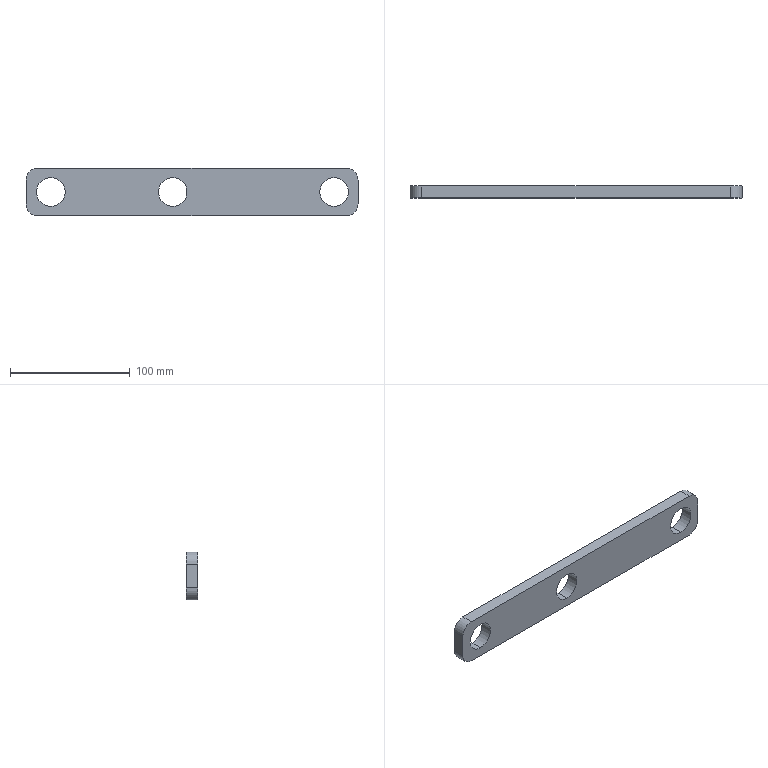Part | SolidWorks | features Extrusion 1, Fillet 1, ICE 1 | 1 solid | 16 faces | box 277.743 x 10 x 40 mm | volume 96667 mm3 | cylinder 10 | plane 6 | commonest cylinder face diameters 24 x6 20 x4
STEP:
#1=CARTESIAN_POINT('',(-107.,10.,-12.));
#2=VERTEX_POINT('',#1);
#3=CARTESIAN_POINT('',(-107.,10.,12.));
#4=VERTEX_POINT('',#3);
#5=CARTESIAN_POINT('',(-107.,10.,0.));
#6=DIRECTION('',(0.,1.,0.));
#7=DIRECTION('',(0.,0.,1.));
#8=AXIS2_PLACEMENT_3D('',#5,#6,#7);
#9=CIRCLE('',#8,12.);
#10=EDGE_CURVE('',#2,#4,#9,.T.);
#11=ORIENTED_EDGE('',*,*,#10,.T.);
#12=CARTESIAN_POINT('',(-107.,0.,12.));
#13=VERTEX_POINT('',#12);
#14=CARTESIAN_POINT('',(-107.,10.,12.));
#15=DIRECTION('',(0.,-1.,0.));
#16=VECTOR('',#15,1000.);
#17=LINE('',#14,#16);
#18=EDGE_CURVE('',#4,#13,#17,.T.);
#19=ORIENTED_EDGE('',*,*,#18,.T.);
#20=CARTESIAN_POINT('',(-107.,0.,-12.));
#21=VERTEX_POINT('',#20);
#22=CARTESIAN_POINT('',(-107.,0.,0.));
#23=DIRECTION('',(0.,1.,0.));
#24=DIRECTION('',(0.,0.,1.));
#25=AXIS2_PLACEMENT_3D('',#22,#23,#24);
#26=CIRCLE('',#25,12.);
#27=EDGE_CURVE('',#21,#13,#26,.T.);
#28=ORIENTED_EDGE('',*,*,#27,.F.);
#29=CARTESIAN_POINT('',(-107.,10.,-12.));
#30=DIRECTION('',(0.,-1.,0.));
#31=VECTOR('',#30,1000.);
#32=LINE('',#29,#31);
#33=EDGE_CURVE('',#2,#21,#32,.T.);
#34=ORIENTED_EDGE('',*,*,#33,.F.);
#35=EDGE_LOOP('',(#11,#19,#28,#34));
#36=FACE_OUTER_BOUND('',#35,.T.);
#37=CARTESIAN_POINT('',(-107.,10.,0.));
#38=DIRECTION('',(0.,-1.,0.));
#39=DIRECTION('',(0.,0.,-1.));
#40=AXIS2_PLACEMENT_3D('',#37,#38,#39);
#41=CYLINDRICAL_SURFACE('',#40,12.);
#42=ADVANCED_FACE('',(#36),#41,.F.);
#43=CARTESIAN_POINT('',(-5.,10.,-12.));
#44=VERTEX_POINT('',#43);
#45=CARTESIAN_POINT('',(-5.,10.,12.));
#46=VERTEX_POINT('',#45);
#47=CARTESIAN_POINT('',(-5.,10.,0.));
#48=DIRECTION('',(0.,1.,0.));
#49=DIRECTION('',(0.,0.,1.));
#50=AXIS2_PLACEMENT_3D('',#47,#48,#49);
#51=CIRCLE('',#50,12.);
#52=EDGE_CURVE('',#44,#46,#51,.T.);
#53=ORIENTED_EDGE('',*,*,#52,.T.);
#54=CARTESIAN_POINT('',(-5.,0.,12.));
#55=VERTEX_POINT('',#54);
#56=CARTESIAN_POINT('',(-5.,10.,12.));
#57=DIRECTION('',(0.,-1.,0.));
#58=VECTOR('',#57,1000.);
#59=LINE('',#56,#58);
#60=EDGE_CURVE('',#46,#55,#59,.T.);
#61=ORIENTED_EDGE('',*,*,#60,.T.);
#62=CARTESIAN_POINT('',(-5.,0.,-12.));
#63=VERTEX_POINT('',#62);
#64=CARTESIAN_POINT('',(-5.,0.,0.));
#65=DIRECTION('',(0.,1.,0.));
#66=DIRECTION('',(0.,0.,1.));
#67=AXIS2_PLACEMENT_3D('',#64,#65,#66);
#68=CIRCLE('',#67,12.);
#69=EDGE_CURVE('',#63,#55,#68,.T.);
#70=ORIENTED_EDGE('',*,*,#69,.F.);
#71=CARTESIAN_POINT('',(-5.,10.,-12.));
#72=DIRECTION('',(0.,-1.,0.));
#73=VECTOR('',#72,1000.);
#74=LINE('',#71,#73);
#75=EDGE_CURVE('',#44,#63,#74,.T.);
#76=ORIENTED_EDGE('',*,*,#75,.F.);
#77=EDGE_LOOP('',(#53,#61,#70,#76));
#78=FACE_OUTER_BOUND('',#77,.T.);
#79=CARTESIAN_POINT('',(-5.,10.,0.));
#80=DIRECTION('',(0.,-1.,0.));
#81=DIRECTION('',(0.,0.,-1.));
#82=AXIS2_PLACEMENT_3D('',#79,#80,#81);
#83=CYLINDRICAL_SURFACE('',#82,12.);
#84=ADVANCED_FACE('',(#78),#83,.F.);
#85=CARTESIAN_POINT('',(130.,10.,-12.));
#86=VERTEX_POINT('',#85);
#87=CARTESIAN_POINT('',(130.,10.,12.));
#88=VERTEX_POINT('',#87);
#89=CARTESIAN_POINT('',(130.,10.,0.));
#90=DIRECTION('',(0.,1.,0.));
#91=DIRECTION('',(0.,0.,1.));
#92=AXIS2_PLACEMENT_3D('',#89,#90,#91);
#93=CIRCLE('',#92,12.);
#94=EDGE_CURVE('',#86,#88,#93,.T.);
#95=ORIENTED_EDGE('',*,*,#94,.T.);
#96=CARTESIAN_POINT('',(130.,0.,12.));
#97=VERTEX_POINT('',#96);
#98=CARTESIAN_POINT('',(130.,10.,12.));
#99=DIRECTION('',(0.,-1.,0.));
#100=VECTOR('',#99,1000.);
#101=LINE('',#98,#100);
#102=EDGE_CURVE('',#88,#97,#101,.T.);
#103=ORIENTED_EDGE('',*,*,#102,.T.);
#104=CARTESIAN_POINT('',(130.,0.,-12.));
#105=VERTEX_POINT('',#104);
#106=CARTESIAN_POINT('',(130.,0.,0.));
#107=DIRECTION('',(0.,1.,0.));
#108=DIRECTION('',(0.,0.,1.));
#109=AXIS2_PLACEMENT_3D('',#106,#107,#108);
#110=CIRCLE('',#109,12.);
#111=EDGE_CURVE('',#105,#97,#110,.T.);
#112=ORIENTED_EDGE('',*,*,#111,.F.);
#113=CARTESIAN_POINT('',(130.,10.,-12.));
#114=DIRECTION('',(0.,-1.,0.));
#115=VECTOR('',#114,1000.);
#116=LINE('',#113,#115);
#117=EDGE_CURVE('',#86,#105,#116,.T.);
#118=ORIENTED_EDGE('',*,*,#117,.F.);
#119=EDGE_LOOP('',(#95,#103,#112,#118));
#120=FACE_OUTER_BOUND('',#119,.T.);
#121=CARTESIAN_POINT('',(130.,10.,0.));
#122=DIRECTION('',(0.,-1.,0.));
#123=DIRECTION('',(0.,0.,-1.));
#124=AXIS2_PLACEMENT_3D('',#121,#122,#123);
#125=CYLINDRICAL_SURFACE('',#124,12.);
#126=ADVANCED_FACE('',(#120),#125,.F.);
#127=CARTESIAN_POINT('',(-117.743,10.,20.));
#128=VERTEX_POINT('',#127);
#129=CARTESIAN_POINT('',(140.,10.,20.));
#130=VERTEX_POINT('',#129);
#131=CARTESIAN_POINT('',(-150.,10.,20.));
#132=DIRECTION('',(1.,0.,0.));
#133=VECTOR('',#132,1000.);
#134=LINE('',#131,#133);
#135=EDGE_CURVE('',#128,#130,#134,.T.);
#136=ORIENTED_EDGE('',*,*,#135,.T.);
#137=CARTESIAN_POINT('',(150.,10.,10.));
#138=VERTEX_POINT('',#137);
#139=CARTESIAN_POINT('',(140.,10.,10.));
#140=DIRECTION('',(0.,1.,0.));
#141=DIRECTION('',(0.,0.,1.));
#142=AXIS2_PLACEMENT_3D('',#139,#140,#141);
#143=CIRCLE('',#142,10.);
#144=EDGE_CURVE('',#130,#138,#143,.T.);
#145=ORIENTED_EDGE('',*,*,#144,.T.);
#146=CARTESIAN_POINT('',(150.,10.,-10.));
#147=VERTEX_POINT('',#146);
#148=CARTESIAN_POINT('',(150.,10.,-20.));
#149=DIRECTION('',(0.,0.,-1.));
#150=VECTOR('',#149,1000.);
#151=LINE('',#148,#150);
#152=EDGE_CURVE('',#138,#147,#151,.T.);
#153=ORIENTED_EDGE('',*,*,#152,.T.);
#154=CARTESIAN_POINT('',(140.,10.,-20.));
#155=VERTEX_POINT('',#154);
#156=CARTESIAN_POINT('',(140.,10.,-10.));
#157=DIRECTION('',(0.,1.,0.));
#158=DIRECTION('',(0.,0.,1.));
#159=AXIS2_PLACEMENT_3D('',#156,#157,#158);
#160=CIRCLE('',#159,10.);
#161=EDGE_CURVE('',#147,#155,#160,.T.);
#162=ORIENTED_EDGE('',*,*,#161,.T.);
#163=CARTESIAN_POINT('',(-117.743,10.,-20.));
#164=VERTEX_POINT('',#163);
#165=CARTESIAN_POINT('',(-150.,10.,-20.));
#166=DIRECTION('',(-1.,0.,0.));
#167=VECTOR('',#166,1000.);
#168=LINE('',#165,#167);
#169=EDGE_CURVE('',#155,#164,#168,.T.);
#170=ORIENTED_EDGE('',*,*,#169,.T.);
#171=CARTESIAN_POINT('',(-127.743,10.,-10.));
#172=VERTEX_POINT('',#171);
#173=CARTESIAN_POINT('',(-117.743,10.,-10.));
#174=DIRECTION('',(0.,1.,0.));
#175=DIRECTION('',(0.,0.,1.));
#176=AXIS2_PLACEMENT_3D('',#173,#174,#175);
#177=CIRCLE('',#176,10.);
#178=EDGE_CURVE('',#164,#172,#177,.T.);
#179=ORIENTED_EDGE('',*,*,#178,.T.);
#180=CARTESIAN_POINT('',(-127.743,10.,10.));
#181=VERTEX_POINT('',#180);
#182=CARTESIAN_POINT('',(-127.743,10.,-20.));
#183=DIRECTION('',(0.,0.,-1.));
#184=VECTOR('',#183,1000.);
#185=LINE('',#182,#184);
#186=EDGE_CURVE('',#181,#172,#185,.T.);
#187=ORIENTED_EDGE('',*,*,#186,.F.);
#188=CARTESIAN_POINT('',(-117.743,10.,10.));
#189=DIRECTION('',(0.,1.,0.));
#190=DIRECTION('',(0.,0.,1.));
#191=AXIS2_PLACEMENT_3D('',#188,#189,#190);
#192=CIRCLE('',#191,10.);
#193=EDGE_CURVE('',#181,#128,#192,.T.);
#194=ORIENTED_EDGE('',*,*,#193,.T.);
#195=EDGE_LOOP('',(#136,#145,#153,#162,#170,#179,#187,#194));
#196=FACE_OUTER_BOUND('',#195,.T.);
#197=ORIENTED_EDGE('',*,*,#52,.F.);
#198=CARTESIAN_POINT('',(-5.,10.,0.));
#199=DIRECTION('',(0.,1.,0.));
#200=DIRECTION('',(0.,0.,1.));
#201=AXIS2_PLACEMENT_3D('',#198,#199,#200);
#202=CIRCLE('',#201,12.);
#203=EDGE_CURVE('',#46,#44,#202,.T.);
#204=ORIENTED_EDGE('',*,*,#203,.F.);
#205=EDGE_LOOP('',(#197,#204));
#206=FACE_BOUND('',#205,.T.);
#207=ORIENTED_EDGE('',*,*,#94,.F.);
#208=CARTESIAN_POINT('',(130.,10.,0.));
#209=DIRECTION('',(0.,1.,0.));
#210=DIRECTION('',(0.,0.,1.));
#211=AXIS2_PLACEMENT_3D('',#208,#209,#210);
#212=CIRCLE('',#211,12.);
#213=EDGE_CURVE('',#88,#86,#212,.T.);
#214=ORIENTED_EDGE('',*,*,#213,.F.);
#215=EDGE_LOOP('',(#207,#214));
#216=FACE_BOUND('',#215,.T.);
#217=ORIENTED_EDGE('',*,*,#10,.F.);
#218=CARTESIAN_POINT('',(-107.,10.,0.));
#219=DIRECTION('',(0.,1.,0.));
#220=DIRECTION('',(0.,0.,1.));
#221=AXIS2_PLACEMENT_3D('',#218,#219,#220);
#222=CIRCLE('',#221,12.);
#223=EDGE_CURVE('',#4,#2,#222,.T.);
#224=ORIENTED_EDGE('',*,*,#223,.F.);
#225=EDGE_LOOP('',(#217,#224));
#226=FACE_BOUND('',#225,.T.);
#227=CARTESIAN_POINT('',(0.,10.,0.));
#228=DIRECTION('',(0.,1.,0.));
#229=DIRECTION('',(0.,0.,1.));
#230=AXIS2_PLACEMENT_3D('',#227,#228,#229);
#231=PLANE('',#230);
#232=ADVANCED_FACE('',(#196,#206,#216,#226),#231,.T.);
#233=CARTESIAN_POINT('',(150.,0.,10.));
#234=VERTEX_POINT('',#233);
#235=CARTESIAN_POINT('',(150.,0.,-10.));
#236=VERTEX_POINT('',#235);
#237=CARTESIAN_POINT('',(150.,0.,-20.));
#238=DIRECTION('',(0.,0.,-1.));
#239=VECTOR('',#238,1000.);
#240=LINE('',#237,#239);
#241=EDGE_CURVE('',#234,#236,#240,.T.);
#242=ORIENTED_EDGE('',*,*,#241,.F.);
#243=CARTESIAN_POINT('',(140.,0.,20.));
#244=VERTEX_POINT('',#243);
#245=CARTESIAN_POINT('',(140.,0.,10.));
#246=DIRECTION('',(0.,-1.,0.));
#247=DIRECTION('',(0.,0.,1.));
#248=AXIS2_PLACEMENT_3D('',#245,#246,#247);
#249=CIRCLE('',#248,10.);
#250=EDGE_CURVE('',#234,#244,#249,.T.);
#251=ORIENTED_EDGE('',*,*,#250,.T.);
#252=CARTESIAN_POINT('',(-117.743,0.,20.));
#253=VERTEX_POINT('',#252);
#254=CARTESIAN_POINT('',(-150.,0.,20.));
#255=DIRECTION('',(1.,0.,0.));
#256=VECTOR('',#255,1000.);
#257=LINE('',#254,#256);
#258=EDGE_CURVE('',#253,#244,#257,.T.);
#259=ORIENTED_EDGE('',*,*,#258,.F.);
#260=CARTESIAN_POINT('',(-127.743,0.,10.));
#261=VERTEX_POINT('',#260);
#262=CARTESIAN_POINT('',(-117.743,0.,10.));
#263=DIRECTION('',(0.,-1.,0.));
#264=DIRECTION('',(0.,0.,1.));
#265=AXIS2_PLACEMENT_3D('',#262,#263,#264);
#266=CIRCLE('',#265,10.);
#267=EDGE_CURVE('',#253,#261,#266,.T.);
#268=ORIENTED_EDGE('',*,*,#267,.T.);
#269=CARTESIAN_POINT('',(-127.743,0.,-10.));
#270=VERTEX_POINT('',#269);
#271=CARTESIAN_POINT('',(-127.743,0.,-20.));
#272=DIRECTION('',(0.,0.,-1.));
#273=VECTOR('',#272,1000.);
#274=LINE('',#271,#273);
#275=EDGE_CURVE('',#261,#270,#274,.T.);
#276=ORIENTED_EDGE('',*,*,#275,.T.);
#277=CARTESIAN_POINT('',(-117.743,0.,-20.));
#278=VERTEX_POINT('',#277);
#279=CARTESIAN_POINT('',(-117.743,0.,-10.));
#280=DIRECTION('',(0.,-1.,0.));
#281=DIRECTION('',(0.,0.,1.));
#282=AXIS2_PLACEMENT_3D('',#279,#280,#281);
#283=CIRCLE('',#282,10.);
#284=EDGE_CURVE('',#270,#278,#283,.T.);
#285=ORIENTED_EDGE('',*,*,#284,.T.);
#286=CARTESIAN_POINT('',(140.,0.,-20.));
#287=VERTEX_POINT('',#286);
#288=CARTESIAN_POINT('',(-150.,0.,-20.));
#289=DIRECTION('',(-1.,0.,0.));
#290=VECTOR('',#289,1000.);
#291=LINE('',#288,#290);
#292=EDGE_CURVE('',#287,#278,#291,.T.);
#293=ORIENTED_EDGE('',*,*,#292,.F.);
#294=CARTESIAN_POINT('',(140.,0.,-10.));
#295=DIRECTION('',(0.,-1.,0.));
#296=DIRECTION('',(0.,0.,1.));
#297=AXIS2_PLACEMENT_3D('',#294,#295,#296);
#298=CIRCLE('',#297,10.);
#299=EDGE_CURVE('',#287,#236,#298,.T.);
#300=ORIENTED_EDGE('',*,*,#299,.T.);
#301=EDGE_LOOP('',(#242,#251,#259,#268,#276,#285,#293,#300));
#302=FACE_OUTER_BOUND('',#301,.T.);
#303=ORIENTED_EDGE('',*,*,#111,.T.);
#304=CARTESIAN_POINT('',(130.,0.,0.));
#305=DIRECTION('',(0.,1.,0.));
#306=DIRECTION('',(0.,0.,1.));
#307=AXIS2_PLACEMENT_3D('',#304,#305,#306);
#308=CIRCLE('',#307,12.);
#309=EDGE_CURVE('',#97,#105,#308,.T.);
#310=ORIENTED_EDGE('',*,*,#309,.T.);
#311=EDGE_LOOP('',(#303,#310));
#312=FACE_BOUND('',#311,.T.);
#313=ORIENTED_EDGE('',*,*,#69,.T.);
#314=CARTESIAN_POINT('',(-5.,0.,0.));
#315=DIRECTION('',(0.,1.,0.));
#316=DIRECTION('',(0.,0.,1.));
#317=AXIS2_PLACEMENT_3D('',#314,#315,#316);
#318=CIRCLE('',#317,12.);
#319=EDGE_CURVE('',#55,#63,#318,.T.);
#320=ORIENTED_EDGE('',*,*,#319,.T.);
#321=EDGE_LOOP('',(#313,#320));
#322=FACE_BOUND('',#321,.T.);
#323=ORIENTED_EDGE('',*,*,#27,.T.);
#324=CARTESIAN_POINT('',(-107.,0.,0.));
#325=DIRECTION('',(0.,1.,0.));
#326=DIRECTION('',(0.,0.,1.));
#327=AXIS2_PLACEMENT_3D('',#324,#325,#326);
#328=CIRCLE('',#327,12.);
#329=EDGE_CURVE('',#13,#21,#328,.T.);
#330=ORIENTED_EDGE('',*,*,#329,.T.);
#331=EDGE_LOOP('',(#323,#330));
#332=FACE_BOUND('',#331,.T.);
#333=CARTESIAN_POINT('',(0.,0.,0.));
#334=DIRECTION('',(0.,1.,0.));
#335=DIRECTION('',(0.,0.,1.));
#336=AXIS2_PLACEMENT_3D('',#333,#334,#335);
#337=PLANE('',#336);
#338=ADVANCED_FACE('',(#302,#312,#322,#332),#337,.F.);
#339=ORIENTED_EDGE('',*,*,#152,.F.);
#340=CARTESIAN_POINT('',(150.,10.,10.));
#341=DIRECTION('',(0.,-1.,0.));
#342=VECTOR('',#341,1000.);
#343=LINE('',#340,#342);
#344=EDGE_CURVE('',#138,#234,#343,.T.);
#345=ORIENTED_EDGE('',*,*,#344,.T.);
#346=ORIENTED_EDGE('',*,*,#241,.T.);
#347=CARTESIAN_POINT('',(150.,10.,-10.));
#348=DIRECTION('',(0.,1.,0.));
#349=VECTOR('',#348,1000.);
#350=LINE('',#347,#349);
#351=EDGE_CURVE('',#236,#147,#350,.T.);
#352=ORIENTED_EDGE('',*,*,#351,.T.);
#353=EDGE_LOOP('',(#339,#345,#346,#352));
#354=FACE_OUTER_BOUND('',#353,.T.);
#355=CARTESIAN_POINT('',(150.,10.,-20.));
#356=DIRECTION('',(-1.,0.,0.));
#357=DIRECTION('',(0.,0.,1.));
#358=AXIS2_PLACEMENT_3D('',#355,#356,#357);
#359=PLANE('',#358);
#360=ADVANCED_FACE('',(#354),#359,.F.);
#361=ORIENTED_EDGE('',*,*,#169,.F.);
#362=CARTESIAN_POINT('',(140.,10.,-20.));
#363=DIRECTION('',(0.,-1.,0.));
#364=VECTOR('',#363,1000.);
#365=LINE('',#362,#364);
#366=EDGE_CURVE('',#155,#287,#365,.T.);
#367=ORIENTED_EDGE('',*,*,#366,.T.);
#368=ORIENTED_EDGE('',*,*,#292,.T.);
#369=CARTESIAN_POINT('',(-117.743,10.,-20.));
#370=DIRECTION('',(0.,1.,0.));
#371=VECTOR('',#370,1000.);
#372=LINE('',#369,#371);
#373=EDGE_CURVE('',#278,#164,#372,.T.);
#374=ORIENTED_EDGE('',*,*,#373,.T.);
#375=EDGE_LOOP('',(#361,#367,#368,#374));
#376=FACE_OUTER_BOUND('',#375,.T.);
#377=CARTESIAN_POINT('',(-150.,10.,-20.));
#378=DIRECTION('',(0.,0.,1.));
#379=DIRECTION('',(1.,0.,0.));
#380=AXIS2_PLACEMENT_3D('',#377,#378,#379);
#381=PLANE('',#380);
#382=ADVANCED_FACE('',(#376),#381,.F.);
#383=ORIENTED_EDGE('',*,*,#258,.T.);
#384=CARTESIAN_POINT('',(140.,10.,20.));
#385=DIRECTION('',(0.,1.,0.));
#386=VECTOR('',#385,1000.);
#387=LINE('',#384,#386);
#388=EDGE_CURVE('',#244,#130,#387,.T.);
#389=ORIENTED_EDGE('',*,*,#388,.T.);
#390=ORIENTED_EDGE('',*,*,#135,.F.);
#391=CARTESIAN_POINT('',(-117.743,10.,20.));
#392=DIRECTION('',(0.,-1.,0.));
#393=VECTOR('',#392,1000.);
#394=LINE('',#391,#393);
#395=EDGE_CURVE('',#128,#253,#394,.T.);
#396=ORIENTED_EDGE('',*,*,#395,.T.);
#397=EDGE_LOOP('',(#383,#389,#390,#396));
#398=FACE_OUTER_BOUND('',#397,.T.);
#399=CARTESIAN_POINT('',(-150.,10.,20.));
#400=DIRECTION('',(0.,0.,-1.));
#401=DIRECTION('',(-1.,0.,0.));
#402=AXIS2_PLACEMENT_3D('',#399,#400,#401);
#403=PLANE('',#402);
#404=ADVANCED_FACE('',(#398),#403,.F.);
#405=ORIENTED_EDGE('',*,*,#102,.F.);
#406=ORIENTED_EDGE('',*,*,#213,.T.);
#407=ORIENTED_EDGE('',*,*,#117,.T.);
#408=ORIENTED_EDGE('',*,*,#309,.F.);
#409=EDGE_LOOP('',(#405,#406,#407,#408));
#410=FACE_OUTER_BOUND('',#409,.T.);
#411=CARTESIAN_POINT('',(130.,10.,0.));
#412=DIRECTION('',(0.,-1.,0.));
#413=DIRECTION('',(0.,0.,-1.));
#414=AXIS2_PLACEMENT_3D('',#411,#412,#413);
#415=CYLINDRICAL_SURFACE('',#414,12.);
#416=ADVANCED_FACE('',(#410),#415,.F.);
#417=ORIENTED_EDGE('',*,*,#60,.F.);
#418=ORIENTED_EDGE('',*,*,#203,.T.);
#419=ORIENTED_EDGE('',*,*,#75,.T.);
#420=ORIENTED_EDGE('',*,*,#319,.F.);
#421=EDGE_LOOP('',(#417,#418,#419,#420));
#422=FACE_OUTER_BOUND('',#421,.T.);
#423=CARTESIAN_POINT('',(-5.,10.,0.));
#424=DIRECTION('',(0.,-1.,0.));
#425=DIRECTION('',(0.,0.,-1.));
#426=AXIS2_PLACEMENT_3D('',#423,#424,#425);
#427=CYLINDRICAL_SURFACE('',#426,12.);
#428=ADVANCED_FACE('',(#422),#427,.F.);
#429=ORIENTED_EDGE('',*,*,#18,.F.);
#430=ORIENTED_EDGE('',*,*,#223,.T.);
#431=ORIENTED_EDGE('',*,*,#33,.T.);
#432=ORIENTED_EDGE('',*,*,#329,.F.);
#433=EDGE_LOOP('',(#429,#430,#431,#432));
#434=FACE_OUTER_BOUND('',#433,.T.);
#435=CARTESIAN_POINT('',(-107.,10.,0.));
#436=DIRECTION('',(0.,-1.,0.));
#437=DIRECTION('',(0.,0.,-1.));
#438=AXIS2_PLACEMENT_3D('',#435,#436,#437);
#439=CYLINDRICAL_SURFACE('',#438,12.);
#440=ADVANCED_FACE('',(#434),#439,.F.);
#441=ORIENTED_EDGE('',*,*,#275,.F.);
#442=CARTESIAN_POINT('',(-127.743,0.,10.));
#443=DIRECTION('',(0.,1.,0.));
#444=VECTOR('',#443,1000.);
#445=LINE('',#442,#444);
#446=EDGE_CURVE('',#261,#181,#445,.T.);
#447=ORIENTED_EDGE('',*,*,#446,.T.);
#448=ORIENTED_EDGE('',*,*,#186,.T.);
#449=CARTESIAN_POINT('',(-127.743,0.,-10.));
#450=DIRECTION('',(0.,-1.,0.));
#451=VECTOR('',#450,1000.);
#452=LINE('',#449,#451);
#453=EDGE_CURVE('',#172,#270,#452,.T.);
#454=ORIENTED_EDGE('',*,*,#453,.T.);
#455=EDGE_LOOP('',(#441,#447,#448,#454));
#456=FACE_OUTER_BOUND('',#455,.T.);
#457=CARTESIAN_POINT('',(-127.743,0.,-20.));
#458=DIRECTION('',(1.,0.,0.));
#459=DIRECTION('',(0.,0.,-1.));
#460=AXIS2_PLACEMENT_3D('',#457,#458,#459);
#461=PLANE('',#460);
#462=ADVANCED_FACE('',(#456),#461,.F.);
#463=ORIENTED_EDGE('',*,*,#144,.F.);
#464=ORIENTED_EDGE('',*,*,#388,.F.);
#465=ORIENTED_EDGE('',*,*,#250,.F.);
#466=ORIENTED_EDGE('',*,*,#344,.F.);
#467=EDGE_LOOP('',(#463,#464,#465,#466));
#468=FACE_OUTER_BOUND('',#467,.T.);
#469=CARTESIAN_POINT('',(140.,10.,10.));
#470=DIRECTION('',(0.,-1.,0.));
#471=DIRECTION('',(0.,0.,-1.));
#472=AXIS2_PLACEMENT_3D('',#469,#470,#471);
#473=CYLINDRICAL_SURFACE('',#472,10.);
#474=ADVANCED_FACE('',(#468),#473,.T.);
#475=ORIENTED_EDGE('',*,*,#161,.F.);
#476=ORIENTED_EDGE('',*,*,#351,.F.);
#477=ORIENTED_EDGE('',*,*,#299,.F.);
#478=ORIENTED_EDGE('',*,*,#366,.F.);
#479=EDGE_LOOP('',(#475,#476,#477,#478));
#480=FACE_OUTER_BOUND('',#479,.T.);
#481=CARTESIAN_POINT('',(140.,10.,-10.));
#482=DIRECTION('',(0.,-1.,0.));
#483=DIRECTION('',(0.,0.,-1.));
#484=AXIS2_PLACEMENT_3D('',#481,#482,#483);
#485=CYLINDRICAL_SURFACE('',#484,10.);
#486=ADVANCED_FACE('',(#480),#485,.T.);
#487=ORIENTED_EDGE('',*,*,#267,.F.);
#488=ORIENTED_EDGE('',*,*,#395,.F.);
#489=ORIENTED_EDGE('',*,*,#193,.F.);
#490=ORIENTED_EDGE('',*,*,#446,.F.);
#491=EDGE_LOOP('',(#487,#488,#489,#490));
#492=FACE_OUTER_BOUND('',#491,.T.);
#493=CARTESIAN_POINT('',(-117.743,0.,10.));
#494=DIRECTION('',(0.,1.,0.));
#495=DIRECTION('',(0.,0.,1.));
#496=AXIS2_PLACEMENT_3D('',#493,#494,#495);
#497=CYLINDRICAL_SURFACE('',#496,10.);
#498=ADVANCED_FACE('',(#492),#497,.T.);
#499=ORIENTED_EDGE('',*,*,#284,.F.);
#500=ORIENTED_EDGE('',*,*,#453,.F.);
#501=ORIENTED_EDGE('',*,*,#178,.F.);
#502=ORIENTED_EDGE('',*,*,#373,.F.);
#503=EDGE_LOOP('',(#499,#500,#501,#502));
#504=FACE_OUTER_BOUND('',#503,.T.);
#505=CARTESIAN_POINT('',(-117.743,10.,-10.));
#506=DIRECTION('',(0.,1.,0.));
#507=DIRECTION('',(0.,0.,1.));
#508=AXIS2_PLACEMENT_3D('',#505,#506,#507);
#509=CYLINDRICAL_SURFACE('',#508,10.);
#510=ADVANCED_FACE('',(#504),#509,.T.);
#511=CLOSED_SHELL('',(#42,#84,#126,#232,#338,#360,#382,#404,#416,#428,#440,#462,#474,#486,#498,#510));
#512=MANIFOLD_SOLID_BREP('',#511);
#513=CARTESIAN_POINT('',(0.,0.,0.));
#514=DIRECTION('',(0.,0.,1.));
#515=DIRECTION('',(1.,0.,0.));
#516=AXIS2_PLACEMENT_3D('',#513,#514,#515);
#517=(LENGTH_UNIT()NAMED_UNIT(*)SI_UNIT(.MILLI.,.METRE.));
#518=UNCERTAINTY_MEASURE_WITH_UNIT(LENGTH_MEASURE(0.00001),#517,'','');
#519=(NAMED_UNIT(*)PLANE_ANGLE_UNIT()SI_UNIT($,.RADIAN.));
#520=(NAMED_UNIT(*)SI_UNIT($,.STERADIAN.)SOLID_ANGLE_UNIT());
#521=(GEOMETRIC_REPRESENTATION_CONTEXT(3)GLOBAL_UNCERTAINTY_ASSIGNED_CONTEXT((#518))GLOBAL_UNIT_ASSIGNED_CONTEXT((#517,#519,#520))REPRESENTATION_CONTEXT('',''));
#522=ADVANCED_BREP_SHAPE_REPRESENTATION('',(#512,#516),#521);